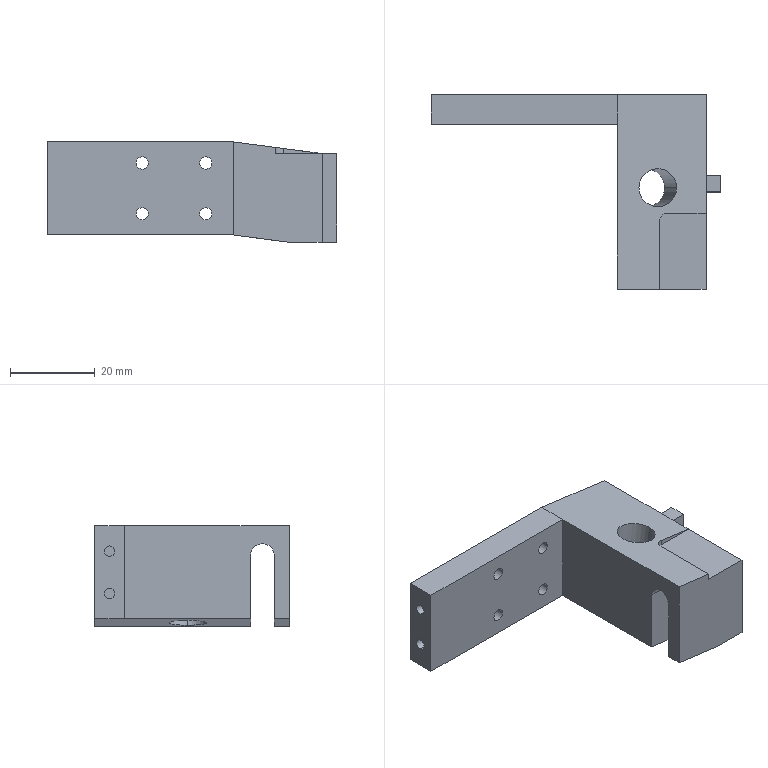Part | SolidWorks | features ICE 9, Extrusion 1 | 1 solid | 56 faces | box 68.5 x 46 x 23.69 mm | volume 23903 mm3 | plane 30 | cylinder 26 | commonest cylinder face diameters 2.9 x8 5 x8 2.5 x4 4.5 x2 9 x2 4 x1